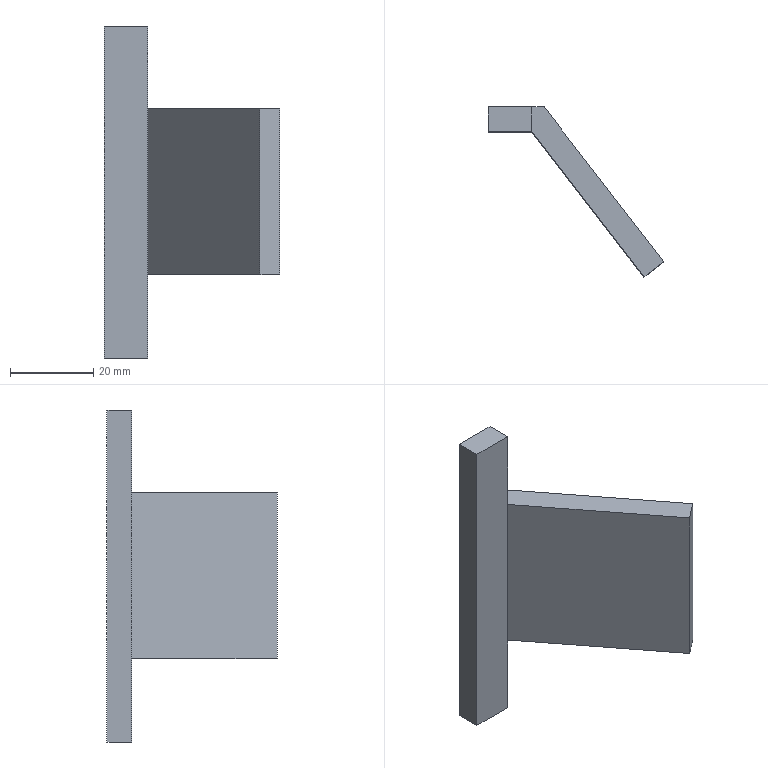Part | SolidWorks | features Extrusion 1, ICE 1, MirrorPattern 1 | 1 solid | 12 faces | box 42.25 x 40.996 x 80 mm | volume 16356 mm3 | plane 12
STEP:
#1=CARTESIAN_POINT('',(10.5,0.,-20.));
#2=VERTEX_POINT('',#1);
#3=CARTESIAN_POINT('',(37.499,-34.996,-20.));
#4=VERTEX_POINT('',#3);
#5=CARTESIAN_POINT('',(10.5,0.,-20.));
#6=DIRECTION('',(0.6108,-0.7918,0.));
#7=VECTOR('',#6,1000.);
#8=LINE('',#5,#7);
#9=EDGE_CURVE('',#2,#4,#8,.T.);
#10=ORIENTED_EDGE('',*,*,#9,.F.);
#11=CARTESIAN_POINT('',(10.5,6.,-20.));
#12=VERTEX_POINT('',#11);
#13=CARTESIAN_POINT('',(10.5,6.,-20.));
#14=DIRECTION('',(0.,1.,0.));
#15=VECTOR('',#14,1000.);
#16=LINE('',#13,#15);
#17=EDGE_CURVE('',#2,#12,#16,.T.);
#18=ORIENTED_EDGE('',*,*,#17,.T.);
#19=CARTESIAN_POINT('',(13.449,6.,-20.));
#20=VERTEX_POINT('',#19);
#21=CARTESIAN_POINT('',(0.,6.,-20.));
#22=DIRECTION('',(-1.,0.,0.));
#23=VECTOR('',#22,1000.);
#24=LINE('',#21,#23);
#25=EDGE_CURVE('',#20,#12,#24,.T.);
#26=ORIENTED_EDGE('',*,*,#25,.F.);
#27=CARTESIAN_POINT('',(42.25,-31.331,-20.));
#28=VERTEX_POINT('',#27);
#29=CARTESIAN_POINT('',(13.449,6.,-20.));
#30=DIRECTION('',(-0.6108,0.7918,0.));
#31=VECTOR('',#30,1000.);
#32=LINE('',#29,#31);
#33=EDGE_CURVE('',#28,#20,#32,.T.);
#34=ORIENTED_EDGE('',*,*,#33,.F.);
#35=CARTESIAN_POINT('',(37.499,-34.996,-20.));
#36=DIRECTION('',(0.7918,0.6108,0.));
#37=VECTOR('',#36,1000.);
#38=LINE('',#35,#37);
#39=EDGE_CURVE('',#4,#28,#38,.T.);
#40=ORIENTED_EDGE('',*,*,#39,.F.);
#41=EDGE_LOOP('',(#10,#18,#26,#34,#40));
#42=FACE_OUTER_BOUND('',#41,.T.);
#43=CARTESIAN_POINT('',(0.,0.,-20.));
#44=DIRECTION('',(0.,0.,-1.));
#45=DIRECTION('',(-1.,0.,0.));
#46=AXIS2_PLACEMENT_3D('',#43,#44,#45);
#47=PLANE('',#46);
#48=ADVANCED_FACE('',(#42),#47,.T.);
#49=CARTESIAN_POINT('',(10.5,0.,20.));
#50=VERTEX_POINT('',#49);
#51=CARTESIAN_POINT('',(10.5,6.,20.));
#52=VERTEX_POINT('',#51);
#53=CARTESIAN_POINT('',(10.5,6.,20.));
#54=DIRECTION('',(0.,1.,0.));
#55=VECTOR('',#54,1000.);
#56=LINE('',#53,#55);
#57=EDGE_CURVE('',#50,#52,#56,.T.);
#58=ORIENTED_EDGE('',*,*,#57,.F.);
#59=CARTESIAN_POINT('',(37.499,-34.996,20.));
#60=VERTEX_POINT('',#59);
#61=CARTESIAN_POINT('',(10.5,0.,20.));
#62=DIRECTION('',(0.6108,-0.7918,0.));
#63=VECTOR('',#62,1000.);
#64=LINE('',#61,#63);
#65=EDGE_CURVE('',#50,#60,#64,.T.);
#66=ORIENTED_EDGE('',*,*,#65,.T.);
#67=CARTESIAN_POINT('',(42.25,-31.331,20.));
#68=VERTEX_POINT('',#67);
#69=CARTESIAN_POINT('',(37.499,-34.996,20.));
#70=DIRECTION('',(0.7918,0.6108,0.));
#71=VECTOR('',#70,1000.);
#72=LINE('',#69,#71);
#73=EDGE_CURVE('',#60,#68,#72,.T.);
#74=ORIENTED_EDGE('',*,*,#73,.T.);
#75=CARTESIAN_POINT('',(13.449,6.,20.));
#76=VERTEX_POINT('',#75);
#77=CARTESIAN_POINT('',(13.449,6.,20.));
#78=DIRECTION('',(-0.6108,0.7918,0.));
#79=VECTOR('',#78,1000.);
#80=LINE('',#77,#79);
#81=EDGE_CURVE('',#68,#76,#80,.T.);
#82=ORIENTED_EDGE('',*,*,#81,.T.);
#83=CARTESIAN_POINT('',(0.,6.,20.));
#84=DIRECTION('',(-1.,0.,0.));
#85=VECTOR('',#84,1000.);
#86=LINE('',#83,#85);
#87=EDGE_CURVE('',#76,#52,#86,.T.);
#88=ORIENTED_EDGE('',*,*,#87,.T.);
#89=EDGE_LOOP('',(#58,#66,#74,#82,#88));
#90=FACE_OUTER_BOUND('',#89,.T.);
#91=CARTESIAN_POINT('',(0.,0.,20.));
#92=DIRECTION('',(0.,0.,-1.));
#93=DIRECTION('',(-1.,0.,0.));
#94=AXIS2_PLACEMENT_3D('',#91,#92,#93);
#95=PLANE('',#94);
#96=ADVANCED_FACE('',(#90),#95,.F.);
#97=CARTESIAN_POINT('',(0.,6.,40.));
#98=VERTEX_POINT('',#97);
#99=CARTESIAN_POINT('',(0.,6.,-40.));
#100=VERTEX_POINT('',#99);
#101=CARTESIAN_POINT('',(0.,6.,20.));
#102=DIRECTION('',(0.,0.,-1.));
#103=VECTOR('',#102,1000.);
#104=LINE('',#101,#103);
#105=EDGE_CURVE('',#98,#100,#104,.T.);
#106=ORIENTED_EDGE('',*,*,#105,.T.);
#107=CARTESIAN_POINT('',(0.,0.,-40.));
#108=VERTEX_POINT('',#107);
#109=CARTESIAN_POINT('',(0.,6.,-40.));
#110=DIRECTION('',(0.,-1.,0.));
#111=VECTOR('',#110,1000.);
#112=LINE('',#109,#111);
#113=EDGE_CURVE('',#100,#108,#112,.T.);
#114=ORIENTED_EDGE('',*,*,#113,.T.);
#115=CARTESIAN_POINT('',(0.,0.,40.));
#116=VERTEX_POINT('',#115);
#117=CARTESIAN_POINT('',(0.,0.,20.));
#118=DIRECTION('',(0.,0.,-1.));
#119=VECTOR('',#118,1000.);
#120=LINE('',#117,#119);
#121=EDGE_CURVE('',#116,#108,#120,.T.);
#122=ORIENTED_EDGE('',*,*,#121,.F.);
#123=CARTESIAN_POINT('',(0.,6.,40.));
#124=DIRECTION('',(0.,-1.,0.));
#125=VECTOR('',#124,1000.);
#126=LINE('',#123,#125);
#127=EDGE_CURVE('',#98,#116,#126,.T.);
#128=ORIENTED_EDGE('',*,*,#127,.F.);
#129=EDGE_LOOP('',(#106,#114,#122,#128));
#130=FACE_OUTER_BOUND('',#129,.T.);
#131=CARTESIAN_POINT('',(0.,0.,20.));
#132=DIRECTION('',(1.,0.,0.));
#133=DIRECTION('',(0.,0.,-1.));
#134=AXIS2_PLACEMENT_3D('',#131,#132,#133);
#135=PLANE('',#134);
#136=ADVANCED_FACE('',(#130),#135,.F.);
#137=ORIENTED_EDGE('',*,*,#121,.T.);
#138=CARTESIAN_POINT('',(10.5,0.,-40.));
#139=VERTEX_POINT('',#138);
#140=CARTESIAN_POINT('',(0.,0.,-40.));
#141=DIRECTION('',(1.,0.,0.));
#142=VECTOR('',#141,1000.);
#143=LINE('',#140,#142);
#144=EDGE_CURVE('',#108,#139,#143,.T.);
#145=ORIENTED_EDGE('',*,*,#144,.T.);
#146=CARTESIAN_POINT('',(10.5,0.,-40.));
#147=DIRECTION('',(0.,0.,1.));
#148=VECTOR('',#147,1000.);
#149=LINE('',#146,#148);
#150=EDGE_CURVE('',#139,#2,#149,.T.);
#151=ORIENTED_EDGE('',*,*,#150,.T.);
#152=CARTESIAN_POINT('',(10.5,0.,20.));
#153=DIRECTION('',(0.,0.,-1.));
#154=VECTOR('',#153,1000.);
#155=LINE('',#152,#154);
#156=EDGE_CURVE('',#50,#2,#155,.T.);
#157=ORIENTED_EDGE('',*,*,#156,.F.);
#158=CARTESIAN_POINT('',(10.5,0.,40.));
#159=VERTEX_POINT('',#158);
#160=CARTESIAN_POINT('',(10.5,0.,40.));
#161=DIRECTION('',(0.,0.,-1.));
#162=VECTOR('',#161,1000.);
#163=LINE('',#160,#162);
#164=EDGE_CURVE('',#159,#50,#163,.T.);
#165=ORIENTED_EDGE('',*,*,#164,.F.);
#166=CARTESIAN_POINT('',(0.,0.,40.));
#167=DIRECTION('',(1.,0.,0.));
#168=VECTOR('',#167,1000.);
#169=LINE('',#166,#168);
#170=EDGE_CURVE('',#116,#159,#169,.T.);
#171=ORIENTED_EDGE('',*,*,#170,.F.);
#172=EDGE_LOOP('',(#137,#145,#151,#157,#165,#171));
#173=FACE_OUTER_BOUND('',#172,.T.);
#174=CARTESIAN_POINT('',(0.,0.,20.));
#175=DIRECTION('',(0.,1.,0.));
#176=DIRECTION('',(0.,0.,1.));
#177=AXIS2_PLACEMENT_3D('',#174,#175,#176);
#178=PLANE('',#177);
#179=ADVANCED_FACE('',(#173),#178,.F.);
#180=ORIENTED_EDGE('',*,*,#9,.T.);
#181=CARTESIAN_POINT('',(37.499,-34.996,20.));
#182=DIRECTION('',(0.,0.,-1.));
#183=VECTOR('',#182,1000.);
#184=LINE('',#181,#183);
#185=EDGE_CURVE('',#60,#4,#184,.T.);
#186=ORIENTED_EDGE('',*,*,#185,.F.);
#187=ORIENTED_EDGE('',*,*,#65,.F.);
#188=ORIENTED_EDGE('',*,*,#156,.T.);
#189=EDGE_LOOP('',(#180,#186,#187,#188));
#190=FACE_OUTER_BOUND('',#189,.T.);
#191=CARTESIAN_POINT('',(10.5,0.,20.));
#192=DIRECTION('',(0.7918,0.6108,0.));
#193=DIRECTION('',(-0.6108,0.7918,0.));
#194=AXIS2_PLACEMENT_3D('',#191,#192,#193);
#195=PLANE('',#194);
#196=ADVANCED_FACE('',(#190),#195,.F.);
#197=ORIENTED_EDGE('',*,*,#39,.T.);
#198=CARTESIAN_POINT('',(42.25,-31.331,20.));
#199=DIRECTION('',(0.,0.,-1.));
#200=VECTOR('',#199,1000.);
#201=LINE('',#198,#200);
#202=EDGE_CURVE('',#68,#28,#201,.T.);
#203=ORIENTED_EDGE('',*,*,#202,.F.);
#204=ORIENTED_EDGE('',*,*,#73,.F.);
#205=ORIENTED_EDGE('',*,*,#185,.T.);
#206=EDGE_LOOP('',(#197,#203,#204,#205));
#207=FACE_OUTER_BOUND('',#206,.T.);
#208=CARTESIAN_POINT('',(37.499,-34.996,20.));
#209=DIRECTION('',(-0.6108,0.7918,0.));
#210=DIRECTION('',(-0.7918,-0.6108,0.));
#211=AXIS2_PLACEMENT_3D('',#208,#209,#210);
#212=PLANE('',#211);
#213=ADVANCED_FACE('',(#207),#212,.F.);
#214=ORIENTED_EDGE('',*,*,#33,.T.);
#215=CARTESIAN_POINT('',(13.449,6.,20.));
#216=DIRECTION('',(0.,0.,-1.));
#217=VECTOR('',#216,1000.);
#218=LINE('',#215,#217);
#219=EDGE_CURVE('',#76,#20,#218,.T.);
#220=ORIENTED_EDGE('',*,*,#219,.F.);
#221=ORIENTED_EDGE('',*,*,#81,.F.);
#222=ORIENTED_EDGE('',*,*,#202,.T.);
#223=EDGE_LOOP('',(#214,#220,#221,#222));
#224=FACE_OUTER_BOUND('',#223,.T.);
#225=CARTESIAN_POINT('',(13.449,6.,20.));
#226=DIRECTION('',(-0.7918,-0.6108,0.));
#227=DIRECTION('',(0.6108,-0.7918,0.));
#228=AXIS2_PLACEMENT_3D('',#225,#226,#227);
#229=PLANE('',#228);
#230=ADVANCED_FACE('',(#224),#229,.F.);
#231=ORIENTED_EDGE('',*,*,#25,.T.);
#232=CARTESIAN_POINT('',(10.5,6.,-40.));
#233=VERTEX_POINT('',#232);
#234=CARTESIAN_POINT('',(10.5,6.,-40.));
#235=DIRECTION('',(0.,0.,1.));
#236=VECTOR('',#235,1000.);
#237=LINE('',#234,#236);
#238=EDGE_CURVE('',#233,#12,#237,.T.);
#239=ORIENTED_EDGE('',*,*,#238,.F.);
#240=CARTESIAN_POINT('',(0.,6.,-40.));
#241=DIRECTION('',(-1.,0.,0.));
#242=VECTOR('',#241,1000.);
#243=LINE('',#240,#242);
#244=EDGE_CURVE('',#233,#100,#243,.T.);
#245=ORIENTED_EDGE('',*,*,#244,.T.);
#246=ORIENTED_EDGE('',*,*,#105,.F.);
#247=CARTESIAN_POINT('',(10.5,6.,40.));
#248=VERTEX_POINT('',#247);
#249=CARTESIAN_POINT('',(0.,6.,40.));
#250=DIRECTION('',(-1.,0.,0.));
#251=VECTOR('',#250,1000.);
#252=LINE('',#249,#251);
#253=EDGE_CURVE('',#248,#98,#252,.T.);
#254=ORIENTED_EDGE('',*,*,#253,.F.);
#255=CARTESIAN_POINT('',(10.5,6.,40.));
#256=DIRECTION('',(0.,0.,-1.));
#257=VECTOR('',#256,1000.);
#258=LINE('',#255,#257);
#259=EDGE_CURVE('',#248,#52,#258,.T.);
#260=ORIENTED_EDGE('',*,*,#259,.T.);
#261=ORIENTED_EDGE('',*,*,#87,.F.);
#262=ORIENTED_EDGE('',*,*,#219,.T.);
#263=EDGE_LOOP('',(#231,#239,#245,#246,#254,#260,#261,#262));
#264=FACE_OUTER_BOUND('',#263,.T.);
#265=CARTESIAN_POINT('',(0.,6.,20.));
#266=DIRECTION('',(0.,-1.,0.));
#267=DIRECTION('',(0.,0.,-1.));
#268=AXIS2_PLACEMENT_3D('',#265,#266,#267);
#269=PLANE('',#268);
#270=ADVANCED_FACE('',(#264),#269,.F.);
#271=ORIENTED_EDGE('',*,*,#57,.T.);
#272=ORIENTED_EDGE('',*,*,#259,.F.);
#273=CARTESIAN_POINT('',(10.5,6.,40.));
#274=DIRECTION('',(0.,1.,0.));
#275=VECTOR('',#274,1000.);
#276=LINE('',#273,#275);
#277=EDGE_CURVE('',#159,#248,#276,.T.);
#278=ORIENTED_EDGE('',*,*,#277,.F.);
#279=ORIENTED_EDGE('',*,*,#164,.T.);
#280=EDGE_LOOP('',(#271,#272,#278,#279));
#281=FACE_OUTER_BOUND('',#280,.T.);
#282=CARTESIAN_POINT('',(10.5,6.,40.));
#283=DIRECTION('',(-1.,0.,0.));
#284=DIRECTION('',(0.,0.,1.));
#285=AXIS2_PLACEMENT_3D('',#282,#283,#284);
#286=PLANE('',#285);
#287=ADVANCED_FACE('',(#281),#286,.F.);
#288=ORIENTED_EDGE('',*,*,#127,.T.);
#289=ORIENTED_EDGE('',*,*,#170,.T.);
#290=ORIENTED_EDGE('',*,*,#277,.T.);
#291=ORIENTED_EDGE('',*,*,#253,.T.);
#292=EDGE_LOOP('',(#288,#289,#290,#291));
#293=FACE_OUTER_BOUND('',#292,.T.);
#294=CARTESIAN_POINT('',(0.,0.,40.));
#295=DIRECTION('',(0.,0.,1.));
#296=DIRECTION('',(1.,0.,0.));
#297=AXIS2_PLACEMENT_3D('',#294,#295,#296);
#298=PLANE('',#297);
#299=ADVANCED_FACE('',(#293),#298,.T.);
#300=ORIENTED_EDGE('',*,*,#17,.F.);
#301=ORIENTED_EDGE('',*,*,#150,.F.);
#302=CARTESIAN_POINT('',(10.5,6.,-40.));
#303=DIRECTION('',(0.,1.,0.));
#304=VECTOR('',#303,1000.);
#305=LINE('',#302,#304);
#306=EDGE_CURVE('',#139,#233,#305,.T.);
#307=ORIENTED_EDGE('',*,*,#306,.T.);
#308=ORIENTED_EDGE('',*,*,#238,.T.);
#309=EDGE_LOOP('',(#300,#301,#307,#308));
#310=FACE_OUTER_BOUND('',#309,.T.);
#311=CARTESIAN_POINT('',(10.5,6.,-40.));
#312=DIRECTION('',(1.,0.,0.));
#313=DIRECTION('',(0.,0.,-1.));
#314=AXIS2_PLACEMENT_3D('',#311,#312,#313);
#315=PLANE('',#314);
#316=ADVANCED_FACE('',(#310),#315,.T.);
#317=ORIENTED_EDGE('',*,*,#113,.F.);
#318=ORIENTED_EDGE('',*,*,#244,.F.);
#319=ORIENTED_EDGE('',*,*,#306,.F.);
#320=ORIENTED_EDGE('',*,*,#144,.F.);
#321=EDGE_LOOP('',(#317,#318,#319,#320));
#322=FACE_OUTER_BOUND('',#321,.T.);
#323=CARTESIAN_POINT('',(0.,0.,-40.));
#324=DIRECTION('',(0.,0.,-1.));
#325=DIRECTION('',(1.,0.,0.));
#326=AXIS2_PLACEMENT_3D('',#323,#324,#325);
#327=PLANE('',#326);
#328=ADVANCED_FACE('',(#322),#327,.T.);
#329=CLOSED_SHELL('',(#48,#96,#136,#179,#196,#213,#230,#270,#287,#299,#316,#328));
#330=MANIFOLD_SOLID_BREP('',#329);
#331=CARTESIAN_POINT('',(0.,0.,0.));
#332=DIRECTION('',(0.,0.,1.));
#333=DIRECTION('',(1.,0.,0.));
#334=AXIS2_PLACEMENT_3D('',#331,#332,#333);
#335=(LENGTH_UNIT()NAMED_UNIT(*)SI_UNIT(.MILLI.,.METRE.));
#336=UNCERTAINTY_MEASURE_WITH_UNIT(LENGTH_MEASURE(0.00001),#335,'','');
#337=(NAMED_UNIT(*)PLANE_ANGLE_UNIT()SI_UNIT($,.RADIAN.));
#338=(NAMED_UNIT(*)SI_UNIT($,.STERADIAN.)SOLID_ANGLE_UNIT());
#339=(GEOMETRIC_REPRESENTATION_CONTEXT(3)GLOBAL_UNCERTAINTY_ASSIGNED_CONTEXT((#336))GLOBAL_UNIT_ASSIGNED_CONTEXT((#335,#337,#338))REPRESENTATION_CONTEXT('',''));
#340=ADVANCED_BREP_SHAPE_REPRESENTATION('',(#330,#334),#339);